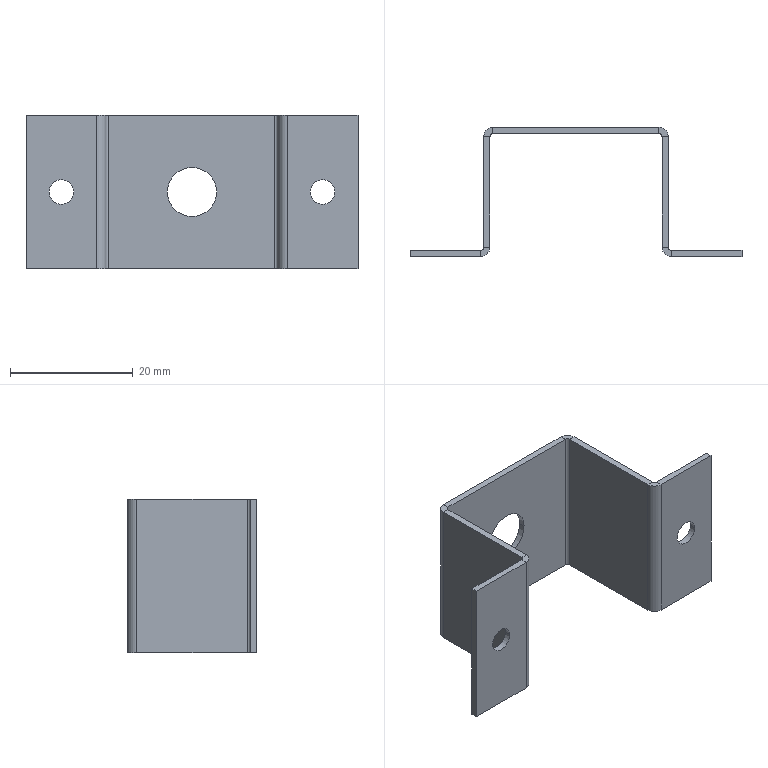Part | SolidWorks | features ICE 2, FlatPattern 1, SMBaseFlange 1, SheetMetal 1 | 1 solid | 44 faces | box 54 x 21 x 25 mm | volume 2232 mm3 | plane 30 | cylinder 14 | commonest cylinder face diameters 1 x4 3 x4 4 x4 8 x2
STEP:
#1=CARTESIAN_POINT('',(23.25,-21.,12.5));
#2=VERTEX_POINT('',#1);
#3=CARTESIAN_POINT('',(19.25,-21.,12.5));
#4=VERTEX_POINT('',#3);
#5=CARTESIAN_POINT('',(21.25,-21.,12.5));
#6=DIRECTION('',(0.,1.,0.));
#7=DIRECTION('',(-1.,0.,0.));
#8=AXIS2_PLACEMENT_3D('',#5,#6,#7);
#9=CIRCLE('',#8,2.);
#10=EDGE_CURVE('',#2,#4,#9,.T.);
#11=ORIENTED_EDGE('',*,*,#10,.F.);
#12=CARTESIAN_POINT('',(23.25,-20.,12.5));
#13=VERTEX_POINT('',#12);
#14=CARTESIAN_POINT('',(23.25,-21.,12.5));
#15=DIRECTION('',(0.,1.,0.));
#16=VECTOR('',#15,1000.);
#17=LINE('',#14,#16);
#18=EDGE_CURVE('',#2,#13,#17,.T.);
#19=ORIENTED_EDGE('',*,*,#18,.T.);
#20=CARTESIAN_POINT('',(19.25,-20.,12.5));
#21=VERTEX_POINT('',#20);
#22=CARTESIAN_POINT('',(21.25,-20.,12.5));
#23=DIRECTION('',(0.,1.,0.));
#24=DIRECTION('',(-1.,0.,0.));
#25=AXIS2_PLACEMENT_3D('',#22,#23,#24);
#26=CIRCLE('',#25,2.);
#27=EDGE_CURVE('',#13,#21,#26,.T.);
#28=ORIENTED_EDGE('',*,*,#27,.T.);
#29=CARTESIAN_POINT('',(19.25,-21.,12.5));
#30=DIRECTION('',(0.,1.,0.));
#31=VECTOR('',#30,1000.);
#32=LINE('',#29,#31);
#33=EDGE_CURVE('',#4,#21,#32,.T.);
#34=ORIENTED_EDGE('',*,*,#33,.F.);
#35=EDGE_LOOP('',(#11,#19,#28,#34));
#36=FACE_OUTER_BOUND('',#35,.T.);
#37=CARTESIAN_POINT('',(21.25,-21.,12.5));
#38=DIRECTION('',(0.,1.,0.));
#39=DIRECTION('',(-1.,0.,0.));
#40=AXIS2_PLACEMENT_3D('',#37,#38,#39);
#41=CYLINDRICAL_SURFACE('',#40,2.);
#42=ADVANCED_FACE('',(#36),#41,.F.);
#43=CARTESIAN_POINT('',(-19.25,-21.,12.5));
#44=VERTEX_POINT('',#43);
#45=CARTESIAN_POINT('',(-23.25,-21.,12.5));
#46=VERTEX_POINT('',#45);
#47=CARTESIAN_POINT('',(-21.25,-21.,12.5));
#48=DIRECTION('',(0.,1.,0.));
#49=DIRECTION('',(-1.,0.,0.));
#50=AXIS2_PLACEMENT_3D('',#47,#48,#49);
#51=CIRCLE('',#50,2.);
#52=EDGE_CURVE('',#44,#46,#51,.T.);
#53=ORIENTED_EDGE('',*,*,#52,.F.);
#54=CARTESIAN_POINT('',(-19.25,-20.,12.5));
#55=VERTEX_POINT('',#54);
#56=CARTESIAN_POINT('',(-19.25,-21.,12.5));
#57=DIRECTION('',(0.,1.,0.));
#58=VECTOR('',#57,1000.);
#59=LINE('',#56,#58);
#60=EDGE_CURVE('',#44,#55,#59,.T.);
#61=ORIENTED_EDGE('',*,*,#60,.T.);
#62=CARTESIAN_POINT('',(-23.25,-20.,12.5));
#63=VERTEX_POINT('',#62);
#64=CARTESIAN_POINT('',(-21.25,-20.,12.5));
#65=DIRECTION('',(0.,1.,0.));
#66=DIRECTION('',(-1.,0.,0.));
#67=AXIS2_PLACEMENT_3D('',#64,#65,#66);
#68=CIRCLE('',#67,2.);
#69=EDGE_CURVE('',#55,#63,#68,.T.);
#70=ORIENTED_EDGE('',*,*,#69,.T.);
#71=CARTESIAN_POINT('',(-23.25,-21.,12.5));
#72=DIRECTION('',(0.,1.,0.));
#73=VECTOR('',#72,1000.);
#74=LINE('',#71,#73);
#75=EDGE_CURVE('',#46,#63,#74,.T.);
#76=ORIENTED_EDGE('',*,*,#75,.F.);
#77=EDGE_LOOP('',(#53,#61,#70,#76));
#78=FACE_OUTER_BOUND('',#77,.T.);
#79=CARTESIAN_POINT('',(-21.25,-21.,12.5));
#80=DIRECTION('',(0.,1.,0.));
#81=DIRECTION('',(-1.,0.,0.));
#82=AXIS2_PLACEMENT_3D('',#79,#80,#81);
#83=CYLINDRICAL_SURFACE('',#82,2.);
#84=ADVANCED_FACE('',(#78),#83,.F.);
#85=CARTESIAN_POINT('',(4.,-1.,12.5));
#86=VERTEX_POINT('',#85);
#87=CARTESIAN_POINT('',(-4.,-1.,12.5));
#88=VERTEX_POINT('',#87);
#89=CARTESIAN_POINT('',(0.,-1.,12.5));
#90=DIRECTION('',(0.,1.,0.));
#91=DIRECTION('',(-1.,0.,0.));
#92=AXIS2_PLACEMENT_3D('',#89,#90,#91);
#93=CIRCLE('',#92,4.);
#94=EDGE_CURVE('',#86,#88,#93,.T.);
#95=ORIENTED_EDGE('',*,*,#94,.F.);
#96=CARTESIAN_POINT('',(4.,0.,12.5));
#97=VERTEX_POINT('',#96);
#98=CARTESIAN_POINT('',(4.,-21.,12.5));
#99=DIRECTION('',(0.,1.,0.));
#100=VECTOR('',#99,1000.);
#101=LINE('',#98,#100);
#102=EDGE_CURVE('',#86,#97,#101,.T.);
#103=ORIENTED_EDGE('',*,*,#102,.T.);
#104=CARTESIAN_POINT('',(-4.,0.,12.5));
#105=VERTEX_POINT('',#104);
#106=CARTESIAN_POINT('',(0.,0.,12.5));
#107=DIRECTION('',(0.,1.,0.));
#108=DIRECTION('',(-1.,0.,0.));
#109=AXIS2_PLACEMENT_3D('',#106,#107,#108);
#110=CIRCLE('',#109,4.);
#111=EDGE_CURVE('',#97,#105,#110,.T.);
#112=ORIENTED_EDGE('',*,*,#111,.T.);
#113=CARTESIAN_POINT('',(-4.,-21.,12.5));
#114=DIRECTION('',(0.,1.,0.));
#115=VECTOR('',#114,1000.);
#116=LINE('',#113,#115);
#117=EDGE_CURVE('',#88,#105,#116,.T.);
#118=ORIENTED_EDGE('',*,*,#117,.F.);
#119=EDGE_LOOP('',(#95,#103,#112,#118));
#120=FACE_OUTER_BOUND('',#119,.T.);
#121=CARTESIAN_POINT('',(0.,-21.,12.5));
#122=DIRECTION('',(0.,1.,0.));
#123=DIRECTION('',(-1.,0.,0.));
#124=AXIS2_PLACEMENT_3D('',#121,#122,#123);
#125=CYLINDRICAL_SURFACE('',#124,4.);
#126=ADVANCED_FACE('',(#120),#125,.F.);
#127=CARTESIAN_POINT('',(-15.,-19.5,25.));
#128=VERTEX_POINT('',#127);
#129=CARTESIAN_POINT('',(-14.,-19.5,25.));
#130=VERTEX_POINT('',#129);
#131=CARTESIAN_POINT('',(-15.,-19.5,25.));
#132=DIRECTION('',(1.,0.,0.));
#133=VECTOR('',#132,1000.);
#134=LINE('',#131,#133);
#135=EDGE_CURVE('',#128,#130,#134,.T.);
#136=ORIENTED_EDGE('',*,*,#135,.F.);
#137=CARTESIAN_POINT('',(-15.5,-20.,25.));
#138=VERTEX_POINT('',#137);
#139=CARTESIAN_POINT('',(-15.5,-19.5,25.));
#140=DIRECTION('',(0.,0.,1.));
#141=DIRECTION('',(-1.,0.,0.));
#142=AXIS2_PLACEMENT_3D('',#139,#140,#141);
#143=CIRCLE('',#142,0.5);
#144=EDGE_CURVE('',#138,#128,#143,.T.);
#145=ORIENTED_EDGE('',*,*,#144,.F.);
#146=CARTESIAN_POINT('',(-15.5,-21.,25.));
#147=VERTEX_POINT('',#146);
#148=CARTESIAN_POINT('',(-15.5,-21.,25.));
#149=DIRECTION('',(0.,1.,0.));
#150=VECTOR('',#149,1000.);
#151=LINE('',#148,#150);
#152=EDGE_CURVE('',#147,#138,#151,.T.);
#153=ORIENTED_EDGE('',*,*,#152,.F.);
#154=CARTESIAN_POINT('',(-15.5,-19.5,25.));
#155=DIRECTION('',(0.,0.,1.));
#156=DIRECTION('',(1.,0.,0.));
#157=AXIS2_PLACEMENT_3D('',#154,#155,#156);
#158=CIRCLE('',#157,1.5);
#159=EDGE_CURVE('',#147,#130,#158,.T.);
#160=ORIENTED_EDGE('',*,*,#159,.T.);
#161=EDGE_LOOP('',(#136,#145,#153,#160));
#162=FACE_OUTER_BOUND('',#161,.T.);
#163=CARTESIAN_POINT('',(-15.,-19.5,25.));
#164=DIRECTION('',(0.,0.,1.));
#165=DIRECTION('',(1.,0.,0.));
#166=AXIS2_PLACEMENT_3D('',#163,#164,#165);
#167=PLANE('',#166);
#168=ADVANCED_FACE('',(#162),#167,.T.);
#169=CARTESIAN_POINT('',(-15.,-1.5,25.));
#170=VERTEX_POINT('',#169);
#171=CARTESIAN_POINT('',(-15.,0.,25.));
#172=DIRECTION('',(0.,1.,0.));
#173=VECTOR('',#172,1000.);
#174=LINE('',#171,#173);
#175=EDGE_CURVE('',#128,#170,#174,.T.);
#176=ORIENTED_EDGE('',*,*,#175,.F.);
#177=ORIENTED_EDGE('',*,*,#135,.T.);
#178=CARTESIAN_POINT('',(-14.,-1.5,25.));
#179=VERTEX_POINT('',#178);
#180=CARTESIAN_POINT('',(-14.,0.,25.));
#181=DIRECTION('',(0.,1.,0.));
#182=VECTOR('',#181,1000.);
#183=LINE('',#180,#182);
#184=EDGE_CURVE('',#130,#179,#183,.T.);
#185=ORIENTED_EDGE('',*,*,#184,.T.);
#186=CARTESIAN_POINT('',(-14.,-1.5,25.));
#187=DIRECTION('',(-1.,0.,0.));
#188=VECTOR('',#187,1000.);
#189=LINE('',#186,#188);
#190=EDGE_CURVE('',#179,#170,#189,.T.);
#191=ORIENTED_EDGE('',*,*,#190,.T.);
#192=EDGE_LOOP('',(#176,#177,#185,#191));
#193=FACE_OUTER_BOUND('',#192,.T.);
#194=CARTESIAN_POINT('',(-15.5,-21.,25.));
#195=DIRECTION('',(0.,0.,1.));
#196=DIRECTION('',(1.,0.,0.));
#197=AXIS2_PLACEMENT_3D('',#194,#195,#196);
#198=PLANE('',#197);
#199=ADVANCED_FACE('',(#193),#198,.T.);
#200=CARTESIAN_POINT('',(-15.5,-20.,0.));
#201=VERTEX_POINT('',#200);
#202=CARTESIAN_POINT('',(-15.5,-21.,0.));
#203=VERTEX_POINT('',#202);
#204=CARTESIAN_POINT('',(-15.5,-20.,0.));
#205=DIRECTION('',(0.,-1.,0.));
#206=VECTOR('',#205,1000.);
#207=LINE('',#204,#206);
#208=EDGE_CURVE('',#201,#203,#207,.T.);
#209=ORIENTED_EDGE('',*,*,#208,.F.);
#210=CARTESIAN_POINT('',(-15.,-19.5,0.));
#211=VERTEX_POINT('',#210);
#212=CARTESIAN_POINT('',(-15.5,-19.5,0.));
#213=DIRECTION('',(0.,0.,1.));
#214=DIRECTION('',(-1.,0.,0.));
#215=AXIS2_PLACEMENT_3D('',#212,#213,#214);
#216=CIRCLE('',#215,0.5);
#217=EDGE_CURVE('',#201,#211,#216,.T.);
#218=ORIENTED_EDGE('',*,*,#217,.T.);
#219=CARTESIAN_POINT('',(-14.,-19.5,0.));
#220=VERTEX_POINT('',#219);
#221=CARTESIAN_POINT('',(-14.,-19.5,0.));
#222=DIRECTION('',(-1.,0.,0.));
#223=VECTOR('',#222,1000.);
#224=LINE('',#221,#223);
#225=EDGE_CURVE('',#220,#211,#224,.T.);
#226=ORIENTED_EDGE('',*,*,#225,.F.);
#227=CARTESIAN_POINT('',(-15.5,-19.5,0.));
#228=DIRECTION('',(0.,0.,1.));
#229=DIRECTION('',(1.,0.,0.));
#230=AXIS2_PLACEMENT_3D('',#227,#228,#229);
#231=CIRCLE('',#230,1.5);
#232=EDGE_CURVE('',#203,#220,#231,.T.);
#233=ORIENTED_EDGE('',*,*,#232,.F.);
#234=EDGE_LOOP('',(#209,#218,#226,#233));
#235=FACE_OUTER_BOUND('',#234,.T.);
#236=CARTESIAN_POINT('',(-15.5,-20.,0.));
#237=DIRECTION('',(0.,0.,-1.));
#238=DIRECTION('',(-1.,0.,0.));
#239=AXIS2_PLACEMENT_3D('',#236,#237,#238);
#240=PLANE('',#239);
#241=ADVANCED_FACE('',(#235),#240,.T.);
#242=CARTESIAN_POINT('',(-27.,-20.,0.));
#243=VERTEX_POINT('',#242);
#244=CARTESIAN_POINT('',(-15.,-20.,0.));
#245=DIRECTION('',(1.,0.,0.));
#246=VECTOR('',#245,1000.);
#247=LINE('',#244,#246);
#248=EDGE_CURVE('',#243,#201,#247,.T.);
#249=ORIENTED_EDGE('',*,*,#248,.T.);
#250=ORIENTED_EDGE('',*,*,#208,.T.);
#251=CARTESIAN_POINT('',(-27.,-21.,0.));
#252=VERTEX_POINT('',#251);
#253=CARTESIAN_POINT('',(-15.,-21.,0.));
#254=DIRECTION('',(1.,0.,0.));
#255=VECTOR('',#254,1000.);
#256=LINE('',#253,#255);
#257=EDGE_CURVE('',#252,#203,#256,.T.);
#258=ORIENTED_EDGE('',*,*,#257,.F.);
#259=CARTESIAN_POINT('',(-27.,-21.,0.));
#260=DIRECTION('',(0.,1.,0.));
#261=VECTOR('',#260,1000.);
#262=LINE('',#259,#261);
#263=EDGE_CURVE('',#252,#243,#262,.T.);
#264=ORIENTED_EDGE('',*,*,#263,.T.);
#265=EDGE_LOOP('',(#249,#250,#258,#264));
#266=FACE_OUTER_BOUND('',#265,.T.);
#267=CARTESIAN_POINT('',(-14.,-19.5,0.));
#268=DIRECTION('',(0.,0.,-1.));
#269=DIRECTION('',(-1.,0.,0.));
#270=AXIS2_PLACEMENT_3D('',#267,#268,#269);
#271=PLANE('',#270);
#272=ADVANCED_FACE('',(#266),#271,.T.);
#273=CARTESIAN_POINT('',(-13.5,0.,25.));
#274=VERTEX_POINT('',#273);
#275=CARTESIAN_POINT('',(-13.5,-1.,25.));
#276=VERTEX_POINT('',#275);
#277=CARTESIAN_POINT('',(-13.5,0.,25.));
#278=DIRECTION('',(0.,-1.,0.));
#279=VECTOR('',#278,1000.);
#280=LINE('',#277,#279);
#281=EDGE_CURVE('',#274,#276,#280,.T.);
#282=ORIENTED_EDGE('',*,*,#281,.F.);
#283=CARTESIAN_POINT('',(-13.5,-1.5,25.));
#284=DIRECTION('',(0.,0.,-1.));
#285=DIRECTION('',(1.,0.,0.));
#286=AXIS2_PLACEMENT_3D('',#283,#284,#285);
#287=CIRCLE('',#286,1.5);
#288=EDGE_CURVE('',#170,#274,#287,.T.);
#289=ORIENTED_EDGE('',*,*,#288,.F.);
#290=ORIENTED_EDGE('',*,*,#190,.F.);
#291=CARTESIAN_POINT('',(-13.5,-1.5,25.));
#292=DIRECTION('',(0.,0.,-1.));
#293=DIRECTION('',(1.,0.,0.));
#294=AXIS2_PLACEMENT_3D('',#291,#292,#293);
#295=CIRCLE('',#294,0.5);
#296=EDGE_CURVE('',#179,#276,#295,.T.);
#297=ORIENTED_EDGE('',*,*,#296,.T.);
#298=EDGE_LOOP('',(#282,#289,#290,#297));
#299=FACE_OUTER_BOUND('',#298,.T.);
#300=CARTESIAN_POINT('',(-13.5,0.,25.));
#301=DIRECTION('',(0.,0.,1.));
#302=DIRECTION('',(1.,0.,0.));
#303=AXIS2_PLACEMENT_3D('',#300,#301,#302);
#304=PLANE('',#303);
#305=ADVANCED_FACE('',(#299),#304,.T.);
#306=CARTESIAN_POINT('',(13.5,0.,25.));
#307=VERTEX_POINT('',#306);
#308=CARTESIAN_POINT('',(-15.,0.,25.));
#309=DIRECTION('',(1.,0.,0.));
#310=VECTOR('',#309,1000.);
#311=LINE('',#308,#310);
#312=EDGE_CURVE('',#274,#307,#311,.T.);
#313=ORIENTED_EDGE('',*,*,#312,.F.);
#314=ORIENTED_EDGE('',*,*,#281,.T.);
#315=CARTESIAN_POINT('',(13.5,-1.,25.));
#316=VERTEX_POINT('',#315);
#317=CARTESIAN_POINT('',(-15.,-1.,25.));
#318=DIRECTION('',(1.,0.,0.));
#319=VECTOR('',#318,1000.);
#320=LINE('',#317,#319);
#321=EDGE_CURVE('',#276,#316,#320,.T.);
#322=ORIENTED_EDGE('',*,*,#321,.T.);
#323=CARTESIAN_POINT('',(13.5,-1.,25.));
#324=DIRECTION('',(0.,1.,0.));
#325=VECTOR('',#324,1000.);
#326=LINE('',#323,#325);
#327=EDGE_CURVE('',#316,#307,#326,.T.);
#328=ORIENTED_EDGE('',*,*,#327,.T.);
#329=EDGE_LOOP('',(#313,#314,#322,#328));
#330=FACE_OUTER_BOUND('',#329,.T.);
#331=CARTESIAN_POINT('',(-14.,-1.5,25.));
#332=DIRECTION('',(0.,0.,1.));
#333=DIRECTION('',(1.,0.,0.));
#334=AXIS2_PLACEMENT_3D('',#331,#332,#333);
#335=PLANE('',#334);
#336=ADVANCED_FACE('',(#330),#335,.T.);
#337=CARTESIAN_POINT('',(-15.,-1.5,0.));
#338=VERTEX_POINT('',#337);
#339=CARTESIAN_POINT('',(-14.,-1.5,0.));
#340=VERTEX_POINT('',#339);
#341=CARTESIAN_POINT('',(-15.,-1.5,0.));
#342=DIRECTION('',(1.,0.,0.));
#343=VECTOR('',#342,1000.);
#344=LINE('',#341,#343);
#345=EDGE_CURVE('',#338,#340,#344,.T.);
#346=ORIENTED_EDGE('',*,*,#345,.F.);
#347=CARTESIAN_POINT('',(-13.5,0.,0.));
#348=VERTEX_POINT('',#347);
#349=CARTESIAN_POINT('',(-13.5,-1.5,0.));
#350=DIRECTION('',(0.,0.,-1.));
#351=DIRECTION('',(1.,0.,0.));
#352=AXIS2_PLACEMENT_3D('',#349,#350,#351);
#353=CIRCLE('',#352,1.5);
#354=EDGE_CURVE('',#338,#348,#353,.T.);
#355=ORIENTED_EDGE('',*,*,#354,.T.);
#356=CARTESIAN_POINT('',(-13.5,-1.,0.));
#357=VERTEX_POINT('',#356);
#358=CARTESIAN_POINT('',(-13.5,-1.,0.));
#359=DIRECTION('',(0.,1.,0.));
#360=VECTOR('',#359,1000.);
#361=LINE('',#358,#360);
#362=EDGE_CURVE('',#357,#348,#361,.T.);
#363=ORIENTED_EDGE('',*,*,#362,.F.);
#364=CARTESIAN_POINT('',(-13.5,-1.5,0.));
#365=DIRECTION('',(0.,0.,-1.));
#366=DIRECTION('',(1.,0.,0.));
#367=AXIS2_PLACEMENT_3D('',#364,#365,#366);
#368=CIRCLE('',#367,0.5);
#369=EDGE_CURVE('',#340,#357,#368,.T.);
#370=ORIENTED_EDGE('',*,*,#369,.F.);
#371=EDGE_LOOP('',(#346,#355,#363,#370));
#372=FACE_OUTER_BOUND('',#371,.T.);
#373=CARTESIAN_POINT('',(-15.,-1.5,0.));
#374=DIRECTION('',(0.,0.,-1.));
#375=DIRECTION('',(-1.,0.,0.));
#376=AXIS2_PLACEMENT_3D('',#373,#374,#375);
#377=PLANE('',#376);
#378=ADVANCED_FACE('',(#372),#377,.T.);
#379=CARTESIAN_POINT('',(-15.,0.,0.));
#380=DIRECTION('',(0.,1.,0.));
#381=VECTOR('',#380,1000.);
#382=LINE('',#379,#381);
#383=EDGE_CURVE('',#211,#338,#382,.T.);
#384=ORIENTED_EDGE('',*,*,#383,.T.);
#385=ORIENTED_EDGE('',*,*,#345,.T.);
#386=CARTESIAN_POINT('',(-14.,0.,0.));
#387=DIRECTION('',(0.,1.,0.));
#388=VECTOR('',#387,1000.);
#389=LINE('',#386,#388);
#390=EDGE_CURVE('',#220,#340,#389,.T.);
#391=ORIENTED_EDGE('',*,*,#390,.F.);
#392=ORIENTED_EDGE('',*,*,#225,.T.);
#393=EDGE_LOOP('',(#384,#385,#391,#392));
#394=FACE_OUTER_BOUND('',#393,.T.);
#395=CARTESIAN_POINT('',(-13.5,-1.,0.));
#396=DIRECTION('',(0.,0.,-1.));
#397=DIRECTION('',(-1.,0.,0.));
#398=AXIS2_PLACEMENT_3D('',#395,#396,#397);
#399=PLANE('',#398);
#400=ADVANCED_FACE('',(#394),#399,.T.);
#401=CARTESIAN_POINT('',(15.,-1.5,25.));
#402=VERTEX_POINT('',#401);
#403=CARTESIAN_POINT('',(14.,-1.5,25.));
#404=VERTEX_POINT('',#403);
#405=CARTESIAN_POINT('',(15.,-1.5,25.));
#406=DIRECTION('',(-1.,0.,0.));
#407=VECTOR('',#406,1000.);
#408=LINE('',#405,#407);
#409=EDGE_CURVE('',#402,#404,#408,.T.);
#410=ORIENTED_EDGE('',*,*,#409,.F.);
#411=CARTESIAN_POINT('',(13.5,-1.5,25.));
#412=DIRECTION('',(0.,0.,-1.));
#413=DIRECTION('',(1.,0.,0.));
#414=AXIS2_PLACEMENT_3D('',#411,#412,#413);
#415=CIRCLE('',#414,1.5);
#416=EDGE_CURVE('',#307,#402,#415,.T.);
#417=ORIENTED_EDGE('',*,*,#416,.F.);
#418=ORIENTED_EDGE('',*,*,#327,.F.);
#419=CARTESIAN_POINT('',(13.5,-1.5,25.));
#420=DIRECTION('',(0.,0.,-1.));
#421=DIRECTION('',(1.,0.,0.));
#422=AXIS2_PLACEMENT_3D('',#419,#420,#421);
#423=CIRCLE('',#422,0.5);
#424=EDGE_CURVE('',#316,#404,#423,.T.);
#425=ORIENTED_EDGE('',*,*,#424,.T.);
#426=EDGE_LOOP('',(#410,#417,#418,#425));
#427=FACE_OUTER_BOUND('',#426,.T.);
#428=CARTESIAN_POINT('',(15.,-1.5,25.));
#429=DIRECTION('',(0.,0.,1.));
#430=DIRECTION('',(1.,0.,0.));
#431=AXIS2_PLACEMENT_3D('',#428,#429,#430);
#432=PLANE('',#431);
#433=ADVANCED_FACE('',(#427),#432,.T.);
#434=CARTESIAN_POINT('',(15.,-19.5,25.));
#435=VERTEX_POINT('',#434);
#436=CARTESIAN_POINT('',(15.,0.,25.));
#437=DIRECTION('',(0.,-1.,0.));
#438=VECTOR('',#437,1000.);
#439=LINE('',#436,#438);
#440=EDGE_CURVE('',#402,#435,#439,.T.);
#441=ORIENTED_EDGE('',*,*,#440,.F.);
#442=ORIENTED_EDGE('',*,*,#409,.T.);
#443=CARTESIAN_POINT('',(14.,-19.5,25.));
#444=VERTEX_POINT('',#443);
#445=CARTESIAN_POINT('',(14.,0.,25.));
#446=DIRECTION('',(0.,-1.,0.));
#447=VECTOR('',#446,1000.);
#448=LINE('',#445,#447);
#449=EDGE_CURVE('',#404,#444,#448,.T.);
#450=ORIENTED_EDGE('',*,*,#449,.T.);
#451=CARTESIAN_POINT('',(14.,-19.5,25.));
#452=DIRECTION('',(1.,0.,0.));
#453=VECTOR('',#452,1000.);
#454=LINE('',#451,#453);
#455=EDGE_CURVE('',#444,#435,#454,.T.);
#456=ORIENTED_EDGE('',*,*,#455,.T.);
#457=EDGE_LOOP('',(#441,#442,#450,#456));
#458=FACE_OUTER_BOUND('',#457,.T.);
#459=CARTESIAN_POINT('',(13.5,-1.,25.));
#460=DIRECTION('',(0.,0.,1.));
#461=DIRECTION('',(1.,0.,0.));
#462=AXIS2_PLACEMENT_3D('',#459,#460,#461);
#463=PLANE('',#462);
#464=ADVANCED_FACE('',(#458),#463,.T.);
#465=CARTESIAN_POINT('',(13.5,0.,0.));
#466=VERTEX_POINT('',#465);
#467=CARTESIAN_POINT('',(13.5,-1.,0.));
#468=VERTEX_POINT('',#467);
#469=CARTESIAN_POINT('',(13.5,0.,0.));
#470=DIRECTION('',(0.,-1.,0.));
#471=VECTOR('',#470,1000.);
#472=LINE('',#469,#471);
#473=EDGE_CURVE('',#466,#468,#472,.T.);
#474=ORIENTED_EDGE('',*,*,#473,.F.);
#475=CARTESIAN_POINT('',(15.,-1.5,0.));
#476=VERTEX_POINT('',#475);
#477=CARTESIAN_POINT('',(13.5,-1.5,0.));
#478=DIRECTION('',(0.,0.,-1.));
#479=DIRECTION('',(1.,0.,0.));
#480=AXIS2_PLACEMENT_3D('',#477,#478,#479);
#481=CIRCLE('',#480,1.5);
#482=EDGE_CURVE('',#466,#476,#481,.T.);
#483=ORIENTED_EDGE('',*,*,#482,.T.);
#484=CARTESIAN_POINT('',(14.,-1.5,0.));
#485=VERTEX_POINT('',#484);
#486=CARTESIAN_POINT('',(14.,-1.5,0.));
#487=DIRECTION('',(1.,0.,0.));
#488=VECTOR('',#487,1000.);
#489=LINE('',#486,#488);
#490=EDGE_CURVE('',#485,#476,#489,.T.);
#491=ORIENTED_EDGE('',*,*,#490,.F.);
#492=CARTESIAN_POINT('',(13.5,-1.5,0.));
#493=DIRECTION('',(0.,0.,-1.));
#494=DIRECTION('',(1.,0.,0.));
#495=AXIS2_PLACEMENT_3D('',#492,#493,#494);
#496=CIRCLE('',#495,0.5);
#497=EDGE_CURVE('',#468,#485,#496,.T.);
#498=ORIENTED_EDGE('',*,*,#497,.F.);
#499=EDGE_LOOP('',(#474,#483,#491,#498));
#500=FACE_OUTER_BOUND('',#499,.T.);
#501=CARTESIAN_POINT('',(13.5,0.,0.));
#502=DIRECTION('',(0.,0.,-1.));
#503=DIRECTION('',(-1.,0.,0.));
#504=AXIS2_PLACEMENT_3D('',#501,#502,#503);
#505=PLANE('',#504);
#506=ADVANCED_FACE('',(#500),#505,.T.);
#507=CARTESIAN_POINT('',(-15.,0.,0.));
#508=DIRECTION('',(1.,0.,0.));
#509=VECTOR('',#508,1000.);
#510=LINE('',#507,#509);
#511=EDGE_CURVE('',#348,#466,#510,.T.);
#512=ORIENTED_EDGE('',*,*,#511,.T.);
#513=ORIENTED_EDGE('',*,*,#473,.T.);
#514=CARTESIAN_POINT('',(-15.,-1.,0.));
#515=DIRECTION('',(1.,0.,0.));
#516=VECTOR('',#515,1000.);
#517=LINE('',#514,#516);
#518=EDGE_CURVE('',#357,#468,#517,.T.);
#519=ORIENTED_EDGE('',*,*,#518,.F.);
#520=ORIENTED_EDGE('',*,*,#362,.T.);
#521=EDGE_LOOP('',(#512,#513,#519,#520));
#522=FACE_OUTER_BOUND('',#521,.T.);
#523=CARTESIAN_POINT('',(14.,-1.5,0.));
#524=DIRECTION('',(0.,0.,-1.));
#525=DIRECTION('',(-1.,0.,0.));
#526=AXIS2_PLACEMENT_3D('',#523,#524,#525);
#527=PLANE('',#526);
#528=ADVANCED_FACE('',(#522),#527,.T.);
#529=CARTESIAN_POINT('',(15.5,-20.,25.));
#530=VERTEX_POINT('',#529);
#531=CARTESIAN_POINT('',(15.5,-21.,25.));
#532=VERTEX_POINT('',#531);
#533=CARTESIAN_POINT('',(15.5,-20.,25.));
#534=DIRECTION('',(0.,-1.,0.));
#535=VECTOR('',#534,1000.);
#536=LINE('',#533,#535);
#537=EDGE_CURVE('',#530,#532,#536,.T.);
#538=ORIENTED_EDGE('',*,*,#537,.F.);
#539=CARTESIAN_POINT('',(15.5,-19.5,25.));
#540=DIRECTION('',(0.,0.,1.));
#541=DIRECTION('',(-1.,0.,0.));
#542=AXIS2_PLACEMENT_3D('',#539,#540,#541);
#543=CIRCLE('',#542,0.5);
#544=EDGE_CURVE('',#435,#530,#543,.T.);
#545=ORIENTED_EDGE('',*,*,#544,.F.);
#546=ORIENTED_EDGE('',*,*,#455,.F.);
#547=CARTESIAN_POINT('',(15.5,-19.5,25.));
#548=DIRECTION('',(0.,0.,1.));
#549=DIRECTION('',(1.,0.,0.));
#550=AXIS2_PLACEMENT_3D('',#547,#548,#549);
#551=CIRCLE('',#550,1.5);
#552=EDGE_CURVE('',#444,#532,#551,.T.);
#553=ORIENTED_EDGE('',*,*,#552,.T.);
#554=EDGE_LOOP('',(#538,#545,#546,#553));
#555=FACE_OUTER_BOUND('',#554,.T.);
#556=CARTESIAN_POINT('',(15.5,-20.,25.));
#557=DIRECTION('',(0.,0.,1.));
#558=DIRECTION('',(1.,0.,0.));
#559=AXIS2_PLACEMENT_3D('',#556,#557,#558);
#560=PLANE('',#559);
#561=ADVANCED_FACE('',(#555),#560,.T.);
#562=CARTESIAN_POINT('',(27.,-20.,25.));
#563=VERTEX_POINT('',#562);
#564=CARTESIAN_POINT('',(15.,-20.,25.));
#565=DIRECTION('',(1.,0.,0.));
#566=VECTOR('',#565,1000.);
#567=LINE('',#564,#566);
#568=EDGE_CURVE('',#530,#563,#567,.T.);
#569=ORIENTED_EDGE('',*,*,#568,.F.);
#570=ORIENTED_EDGE('',*,*,#537,.T.);
#571=CARTESIAN_POINT('',(27.,-21.,25.));
#572=VERTEX_POINT('',#571);
#573=CARTESIAN_POINT('',(15.,-21.,25.));
#574=DIRECTION('',(1.,0.,0.));
#575=VECTOR('',#574,1000.);
#576=LINE('',#573,#575);
#577=EDGE_CURVE('',#532,#572,#576,.T.);
#578=ORIENTED_EDGE('',*,*,#577,.T.);
#579=CARTESIAN_POINT('',(27.,-20.,25.));
#580=DIRECTION('',(0.,-1.,0.));
#581=VECTOR('',#580,1000.);
#582=LINE('',#579,#581);
#583=EDGE_CURVE('',#563,#572,#582,.T.);
#584=ORIENTED_EDGE('',*,*,#583,.F.);
#585=EDGE_LOOP('',(#569,#570,#578,#584));
#586=FACE_OUTER_BOUND('',#585,.T.);
#587=CARTESIAN_POINT('',(14.,-19.5,25.));
#588=DIRECTION('',(0.,0.,1.));
#589=DIRECTION('',(1.,0.,0.));
#590=AXIS2_PLACEMENT_3D('',#587,#588,#589);
#591=PLANE('',#590);
#592=ADVANCED_FACE('',(#586),#591,.T.);
#593=CARTESIAN_POINT('',(15.,-19.5,0.));
#594=VERTEX_POINT('',#593);
#595=CARTESIAN_POINT('',(14.,-19.5,0.));
#596=VERTEX_POINT('',#595);
#597=CARTESIAN_POINT('',(15.,-19.5,0.));
#598=DIRECTION('',(-1.,0.,0.));
#599=VECTOR('',#598,1000.);
#600=LINE('',#597,#599);
#601=EDGE_CURVE('',#594,#596,#600,.T.);
#602=ORIENTED_EDGE('',*,*,#601,.F.);
#603=CARTESIAN_POINT('',(15.5,-20.,0.));
#604=VERTEX_POINT('',#603);
#605=CARTESIAN_POINT('',(15.5,-19.5,0.));
#606=DIRECTION('',(0.,0.,1.));
#607=DIRECTION('',(-1.,0.,0.));
#608=AXIS2_PLACEMENT_3D('',#605,#606,#607);
#609=CIRCLE('',#608,0.5);
#610=EDGE_CURVE('',#594,#604,#609,.T.);
#611=ORIENTED_EDGE('',*,*,#610,.T.);
#612=CARTESIAN_POINT('',(15.5,-21.,0.));
#613=VERTEX_POINT('',#612);
#614=CARTESIAN_POINT('',(15.5,-21.,0.));
#615=DIRECTION('',(0.,1.,0.));
#616=VECTOR('',#615,1000.);
#617=LINE('',#614,#616);
#618=EDGE_CURVE('',#613,#604,#617,.T.);
#619=ORIENTED_EDGE('',*,*,#618,.F.);
#620=CARTESIAN_POINT('',(15.5,-19.5,0.));
#621=DIRECTION('',(0.,0.,1.));
#622=DIRECTION('',(1.,0.,0.));
#623=AXIS2_PLACEMENT_3D('',#620,#621,#622);
#624=CIRCLE('',#623,1.5);
#625=EDGE_CURVE('',#596,#613,#624,.T.);
#626=ORIENTED_EDGE('',*,*,#625,.F.);
#627=EDGE_LOOP('',(#602,#611,#619,#626));
#628=FACE_OUTER_BOUND('',#627,.T.);
#629=CARTESIAN_POINT('',(15.,-19.5,0.));
#630=DIRECTION('',(0.,0.,-1.));
#631=DIRECTION('',(-1.,0.,0.));
#632=AXIS2_PLACEMENT_3D('',#629,#630,#631);
#633=PLANE('',#632);
#634=ADVANCED_FACE('',(#628),#633,.T.);
#635=CARTESIAN_POINT('',(15.,0.,0.));
#636=DIRECTION('',(0.,-1.,0.));
#637=VECTOR('',#636,1000.);
#638=LINE('',#635,#637);
#639=EDGE_CURVE('',#476,#594,#638,.T.);
#640=ORIENTED_EDGE('',*,*,#639,.T.);
#641=ORIENTED_EDGE('',*,*,#601,.T.);
#642=CARTESIAN_POINT('',(14.,0.,0.));
#643=DIRECTION('',(0.,-1.,0.));
#644=VECTOR('',#643,1000.);
#645=LINE('',#642,#644);
#646=EDGE_CURVE('',#485,#596,#645,.T.);
#647=ORIENTED_EDGE('',*,*,#646,.F.);
#648=ORIENTED_EDGE('',*,*,#490,.T.);
#649=EDGE_LOOP('',(#640,#641,#647,#648));
#650=FACE_OUTER_BOUND('',#649,.T.);
#651=CARTESIAN_POINT('',(15.5,-21.,0.));
#652=DIRECTION('',(0.,0.,-1.));
#653=DIRECTION('',(-1.,0.,0.));
#654=AXIS2_PLACEMENT_3D('',#651,#652,#653);
#655=PLANE('',#654);
#656=ADVANCED_FACE('',(#650),#655,.T.);
#657=CARTESIAN_POINT('',(21.25,-21.,12.5));
#658=DIRECTION('',(0.,1.,0.));
#659=DIRECTION('',(-1.,0.,0.));
#660=AXIS2_PLACEMENT_3D('',#657,#658,#659);
#661=CIRCLE('',#660,2.);
#662=EDGE_CURVE('',#4,#2,#661,.T.);
#663=ORIENTED_EDGE('',*,*,#662,.T.);
#664=ORIENTED_EDGE('',*,*,#10,.T.);
#665=EDGE_LOOP('',(#663,#664));
#666=FACE_BOUND('',#665,.T.);
#667=CARTESIAN_POINT('',(27.,-21.,0.));
#668=VERTEX_POINT('',#667);
#669=CARTESIAN_POINT('',(15.,-21.,0.));
#670=DIRECTION('',(1.,0.,0.));
#671=VECTOR('',#670,1000.);
#672=LINE('',#669,#671);
#673=EDGE_CURVE('',#613,#668,#672,.T.);
#674=ORIENTED_EDGE('',*,*,#673,.T.);
#675=CARTESIAN_POINT('',(27.,-21.,25.));
#676=DIRECTION('',(0.,0.,-1.));
#677=VECTOR('',#676,1000.);
#678=LINE('',#675,#677);
#679=EDGE_CURVE('',#572,#668,#678,.T.);
#680=ORIENTED_EDGE('',*,*,#679,.F.);
#681=ORIENTED_EDGE('',*,*,#577,.F.);
#682=CARTESIAN_POINT('',(15.5,-21.,25.));
#683=DIRECTION('',(0.,0.,-1.));
#684=VECTOR('',#683,1000.);
#685=LINE('',#682,#684);
#686=EDGE_CURVE('',#532,#613,#685,.T.);
#687=ORIENTED_EDGE('',*,*,#686,.T.);
#688=EDGE_LOOP('',(#674,#680,#681,#687));
#689=FACE_OUTER_BOUND('',#688,.T.);
#690=CARTESIAN_POINT('',(15.,-21.,25.));
#691=DIRECTION('',(0.,1.,0.));
#692=DIRECTION('',(0.,0.,1.));
#693=AXIS2_PLACEMENT_3D('',#690,#691,#692);
#694=PLANE('',#693);
#695=ADVANCED_FACE('',(#666,#689),#694,.F.);
#696=CARTESIAN_POINT('',(27.,-20.,0.));
#697=VERTEX_POINT('',#696);
#698=CARTESIAN_POINT('',(27.,-20.,0.));
#699=DIRECTION('',(0.,-1.,0.));
#700=VECTOR('',#699,1000.);
#701=LINE('',#698,#700);
#702=EDGE_CURVE('',#697,#668,#701,.T.);
#703=ORIENTED_EDGE('',*,*,#702,.F.);
#704=CARTESIAN_POINT('',(27.,-20.,25.));
#705=DIRECTION('',(0.,0.,-1.));
#706=VECTOR('',#705,1000.);
#707=LINE('',#704,#706);
#708=EDGE_CURVE('',#563,#697,#707,.T.);
#709=ORIENTED_EDGE('',*,*,#708,.F.);
#710=ORIENTED_EDGE('',*,*,#583,.T.);
#711=ORIENTED_EDGE('',*,*,#679,.T.);
#712=EDGE_LOOP('',(#703,#709,#710,#711));
#713=FACE_OUTER_BOUND('',#712,.T.);
#714=CARTESIAN_POINT('',(27.,-20.,25.));
#715=DIRECTION('',(1.,0.,0.));
#716=DIRECTION('',(0.,0.,-1.));
#717=AXIS2_PLACEMENT_3D('',#714,#715,#716);
#718=PLANE('',#717);
#719=ADVANCED_FACE('',(#713),#718,.T.);
#720=CARTESIAN_POINT('',(21.25,-20.,12.5));
#721=DIRECTION('',(0.,1.,0.));
#722=DIRECTION('',(-1.,0.,0.));
#723=AXIS2_PLACEMENT_3D('',#720,#721,#722);
#724=CIRCLE('',#723,2.);
#725=EDGE_CURVE('',#21,#13,#724,.T.);
#726=ORIENTED_EDGE('',*,*,#725,.F.);
#727=ORIENTED_EDGE('',*,*,#27,.F.);
#728=EDGE_LOOP('',(#726,#727));
#729=FACE_BOUND('',#728,.T.);
#730=CARTESIAN_POINT('',(15.,-20.,0.));
#731=DIRECTION('',(1.,0.,0.));
#732=VECTOR('',#731,1000.);
#733=LINE('',#730,#732);
#734=EDGE_CURVE('',#604,#697,#733,.T.);
#735=ORIENTED_EDGE('',*,*,#734,.F.);
#736=CARTESIAN_POINT('',(15.5,-20.,25.));
#737=DIRECTION('',(0.,0.,-1.));
#738=VECTOR('',#737,1000.);
#739=LINE('',#736,#738);
#740=EDGE_CURVE('',#530,#604,#739,.T.);
#741=ORIENTED_EDGE('',*,*,#740,.F.);
#742=ORIENTED_EDGE('',*,*,#568,.T.);
#743=ORIENTED_EDGE('',*,*,#708,.T.);
#744=EDGE_LOOP('',(#735,#741,#742,#743));
#745=FACE_OUTER_BOUND('',#744,.T.);
#746=CARTESIAN_POINT('',(15.,-20.,25.));
#747=DIRECTION('',(0.,1.,0.));
#748=DIRECTION('',(0.,0.,1.));
#749=AXIS2_PLACEMENT_3D('',#746,#747,#748);
#750=PLANE('',#749);
#751=ADVANCED_FACE('',(#729,#745),#750,.T.);
#752=ORIENTED_EDGE('',*,*,#610,.F.);
#753=CARTESIAN_POINT('',(15.,-19.5,25.));
#754=DIRECTION('',(0.,0.,-1.));
#755=VECTOR('',#754,1000.);
#756=LINE('',#753,#755);
#757=EDGE_CURVE('',#435,#594,#756,.T.);
#758=ORIENTED_EDGE('',*,*,#757,.F.);
#759=ORIENTED_EDGE('',*,*,#544,.T.);
#760=ORIENTED_EDGE('',*,*,#740,.T.);
#761=EDGE_LOOP('',(#752,#758,#759,#760));
#762=FACE_OUTER_BOUND('',#761,.T.);
#763=CARTESIAN_POINT('',(15.5,-19.5,25.));
#764=DIRECTION('',(0.,0.,-1.));
#765=DIRECTION('',(-1.,0.,0.));
#766=AXIS2_PLACEMENT_3D('',#763,#764,#765);
#767=CYLINDRICAL_SURFACE('',#766,0.5);
#768=ADVANCED_FACE('',(#762),#767,.F.);
#769=ORIENTED_EDGE('',*,*,#639,.F.);
#770=CARTESIAN_POINT('',(15.,-1.5,25.));
#771=DIRECTION('',(0.,0.,-1.));
#772=VECTOR('',#771,1000.);
#773=LINE('',#770,#772);
#774=EDGE_CURVE('',#402,#476,#773,.T.);
#775=ORIENTED_EDGE('',*,*,#774,.F.);
#776=ORIENTED_EDGE('',*,*,#440,.T.);
#777=ORIENTED_EDGE('',*,*,#757,.T.);
#778=EDGE_LOOP('',(#769,#775,#776,#777));
#779=FACE_OUTER_BOUND('',#778,.T.);
#780=CARTESIAN_POINT('',(15.,0.,25.));
#781=DIRECTION('',(1.,0.,0.));
#782=DIRECTION('',(0.,1.,0.));
#783=AXIS2_PLACEMENT_3D('',#780,#781,#782);
#784=PLANE('',#783);
#785=ADVANCED_FACE('',(#779),#784,.T.);
#786=ORIENTED_EDGE('',*,*,#482,.F.);
#787=CARTESIAN_POINT('',(13.5,0.,25.));
#788=DIRECTION('',(0.,0.,-1.));
#789=VECTOR('',#788,1000.);
#790=LINE('',#787,#789);
#791=EDGE_CURVE('',#307,#466,#790,.T.);
#792=ORIENTED_EDGE('',*,*,#791,.F.);
#793=ORIENTED_EDGE('',*,*,#416,.T.);
#794=ORIENTED_EDGE('',*,*,#774,.T.);
#795=EDGE_LOOP('',(#786,#792,#793,#794));
#796=FACE_OUTER_BOUND('',#795,.T.);
#797=CARTESIAN_POINT('',(13.5,-1.5,25.));
#798=DIRECTION('',(0.,0.,-1.));
#799=DIRECTION('',(-1.,0.,0.));
#800=AXIS2_PLACEMENT_3D('',#797,#798,#799);
#801=CYLINDRICAL_SURFACE('',#800,1.5);
#802=ADVANCED_FACE('',(#796),#801,.T.);
#803=CARTESIAN_POINT('',(0.,0.,12.5));
#804=DIRECTION('',(0.,1.,0.));
#805=DIRECTION('',(-1.,0.,0.));
#806=AXIS2_PLACEMENT_3D('',#803,#804,#805);
#807=CIRCLE('',#806,4.);
#808=EDGE_CURVE('',#105,#97,#807,.T.);
#809=ORIENTED_EDGE('',*,*,#808,.F.);
#810=ORIENTED_EDGE('',*,*,#111,.F.);
#811=EDGE_LOOP('',(#809,#810));
#812=FACE_BOUND('',#811,.T.);
#813=ORIENTED_EDGE('',*,*,#511,.F.);
#814=CARTESIAN_POINT('',(-13.5,0.,25.));
#815=DIRECTION('',(0.,0.,-1.));
#816=VECTOR('',#815,1000.);
#817=LINE('',#814,#816);
#818=EDGE_CURVE('',#274,#348,#817,.T.);
#819=ORIENTED_EDGE('',*,*,#818,.F.);
#820=ORIENTED_EDGE('',*,*,#312,.T.);
#821=ORIENTED_EDGE('',*,*,#791,.T.);
#822=EDGE_LOOP('',(#813,#819,#820,#821));
#823=FACE_OUTER_BOUND('',#822,.T.);
#824=CARTESIAN_POINT('',(-15.,0.,25.));
#825=DIRECTION('',(0.,1.,0.));
#826=DIRECTION('',(-1.,0.,0.));
#827=AXIS2_PLACEMENT_3D('',#824,#825,#826);
#828=PLANE('',#827);
#829=ADVANCED_FACE('',(#812,#823),#828,.T.);
#830=ORIENTED_EDGE('',*,*,#354,.F.);
#831=CARTESIAN_POINT('',(-15.,-1.5,25.));
#832=DIRECTION('',(0.,0.,-1.));
#833=VECTOR('',#832,1000.);
#834=LINE('',#831,#833);
#835=EDGE_CURVE('',#170,#338,#834,.T.);
#836=ORIENTED_EDGE('',*,*,#835,.F.);
#837=ORIENTED_EDGE('',*,*,#288,.T.);
#838=ORIENTED_EDGE('',*,*,#818,.T.);
#839=EDGE_LOOP('',(#830,#836,#837,#838));
#840=FACE_OUTER_BOUND('',#839,.T.);
#841=CARTESIAN_POINT('',(-13.5,-1.5,25.));
#842=DIRECTION('',(0.,0.,-1.));
#843=DIRECTION('',(-1.,0.,0.));
#844=AXIS2_PLACEMENT_3D('',#841,#842,#843);
#845=CYLINDRICAL_SURFACE('',#844,1.5);
#846=ADVANCED_FACE('',(#840),#845,.T.);
#847=ORIENTED_EDGE('',*,*,#383,.F.);
#848=CARTESIAN_POINT('',(-15.,-19.5,25.));
#849=DIRECTION('',(0.,0.,-1.));
#850=VECTOR('',#849,1000.);
#851=LINE('',#848,#850);
#852=EDGE_CURVE('',#128,#211,#851,.T.);
#853=ORIENTED_EDGE('',*,*,#852,.F.);
#854=ORIENTED_EDGE('',*,*,#175,.T.);
#855=ORIENTED_EDGE('',*,*,#835,.T.);
#856=EDGE_LOOP('',(#847,#853,#854,#855));
#857=FACE_OUTER_BOUND('',#856,.T.);
#858=CARTESIAN_POINT('',(-15.,0.,25.));
#859=DIRECTION('',(-1.,0.,0.));
#860=DIRECTION('',(0.,-1.,0.));
#861=AXIS2_PLACEMENT_3D('',#858,#859,#860);
#862=PLANE('',#861);
#863=ADVANCED_FACE('',(#857),#862,.T.);
#864=ORIENTED_EDGE('',*,*,#217,.F.);
#865=CARTESIAN_POINT('',(-15.5,-20.,25.));
#866=DIRECTION('',(0.,0.,-1.));
#867=VECTOR('',#866,1000.);
#868=LINE('',#865,#867);
#869=EDGE_CURVE('',#138,#201,#868,.T.);
#870=ORIENTED_EDGE('',*,*,#869,.F.);
#871=ORIENTED_EDGE('',*,*,#144,.T.);
#872=ORIENTED_EDGE('',*,*,#852,.T.);
#873=EDGE_LOOP('',(#864,#870,#871,#872));
#874=FACE_OUTER_BOUND('',#873,.T.);
#875=CARTESIAN_POINT('',(-15.5,-19.5,25.));
#876=DIRECTION('',(0.,0.,-1.));
#877=DIRECTION('',(-1.,0.,0.));
#878=AXIS2_PLACEMENT_3D('',#875,#876,#877);
#879=CYLINDRICAL_SURFACE('',#878,0.5);
#880=ADVANCED_FACE('',(#874),#879,.F.);
#881=CARTESIAN_POINT('',(-21.25,-20.,12.5));
#882=DIRECTION('',(0.,1.,0.));
#883=DIRECTION('',(-1.,0.,0.));
#884=AXIS2_PLACEMENT_3D('',#881,#882,#883);
#885=CIRCLE('',#884,2.);
#886=EDGE_CURVE('',#63,#55,#885,.T.);
#887=ORIENTED_EDGE('',*,*,#886,.F.);
#888=ORIENTED_EDGE('',*,*,#69,.F.);
#889=EDGE_LOOP('',(#887,#888));
#890=FACE_BOUND('',#889,.T.);
#891=ORIENTED_EDGE('',*,*,#248,.F.);
#892=CARTESIAN_POINT('',(-27.,-20.,25.));
#893=VERTEX_POINT('',#892);
#894=CARTESIAN_POINT('',(-27.,-20.,25.));
#895=DIRECTION('',(0.,0.,-1.));
#896=VECTOR('',#895,1000.);
#897=LINE('',#894,#896);
#898=EDGE_CURVE('',#893,#243,#897,.T.);
#899=ORIENTED_EDGE('',*,*,#898,.F.);
#900=CARTESIAN_POINT('',(-15.,-20.,25.));
#901=DIRECTION('',(1.,0.,0.));
#902=VECTOR('',#901,1000.);
#903=LINE('',#900,#902);
#904=EDGE_CURVE('',#893,#138,#903,.T.);
#905=ORIENTED_EDGE('',*,*,#904,.T.);
#906=ORIENTED_EDGE('',*,*,#869,.T.);
#907=EDGE_LOOP('',(#891,#899,#905,#906));
#908=FACE_OUTER_BOUND('',#907,.T.);
#909=CARTESIAN_POINT('',(-15.,-20.,25.));
#910=DIRECTION('',(0.,1.,0.));
#911=DIRECTION('',(-1.,0.,0.));
#912=AXIS2_PLACEMENT_3D('',#909,#910,#911);
#913=PLANE('',#912);
#914=ADVANCED_FACE('',(#890,#908),#913,.T.);
#915=ORIENTED_EDGE('',*,*,#263,.F.);
#916=CARTESIAN_POINT('',(-27.,-21.,25.));
#917=VERTEX_POINT('',#916);
#918=CARTESIAN_POINT('',(-27.,-21.,25.));
#919=DIRECTION('',(0.,0.,-1.));
#920=VECTOR('',#919,1000.);
#921=LINE('',#918,#920);
#922=EDGE_CURVE('',#917,#252,#921,.T.);
#923=ORIENTED_EDGE('',*,*,#922,.F.);
#924=CARTESIAN_POINT('',(-27.,-21.,25.));
#925=DIRECTION('',(0.,1.,0.));
#926=VECTOR('',#925,1000.);
#927=LINE('',#924,#926);
#928=EDGE_CURVE('',#917,#893,#927,.T.);
#929=ORIENTED_EDGE('',*,*,#928,.T.);
#930=ORIENTED_EDGE('',*,*,#898,.T.);
#931=EDGE_LOOP('',(#915,#923,#929,#930));
#932=FACE_OUTER_BOUND('',#931,.T.);
#933=CARTESIAN_POINT('',(-27.,-21.,25.));
#934=DIRECTION('',(-1.,0.,0.));
#935=DIRECTION('',(0.,0.,1.));
#936=AXIS2_PLACEMENT_3D('',#933,#934,#935);
#937=PLANE('',#936);
#938=ADVANCED_FACE('',(#932),#937,.T.);
#939=CARTESIAN_POINT('',(-21.25,-21.,12.5));
#940=DIRECTION('',(0.,1.,0.));
#941=DIRECTION('',(-1.,0.,0.));
#942=AXIS2_PLACEMENT_3D('',#939,#940,#941);
#943=CIRCLE('',#942,2.);
#944=EDGE_CURVE('',#46,#44,#943,.T.);
#945=ORIENTED_EDGE('',*,*,#944,.T.);
#946=ORIENTED_EDGE('',*,*,#52,.T.);
#947=EDGE_LOOP('',(#945,#946));
#948=FACE_BOUND('',#947,.T.);
#949=ORIENTED_EDGE('',*,*,#257,.T.);
#950=CARTESIAN_POINT('',(-15.5,-21.,25.));
#951=DIRECTION('',(0.,0.,-1.));
#952=VECTOR('',#951,1000.);
#953=LINE('',#950,#952);
#954=EDGE_CURVE('',#147,#203,#953,.T.);
#955=ORIENTED_EDGE('',*,*,#954,.F.);
#956=CARTESIAN_POINT('',(-15.,-21.,25.));
#957=DIRECTION('',(1.,0.,0.));
#958=VECTOR('',#957,1000.);
#959=LINE('',#956,#958);
#960=EDGE_CURVE('',#917,#147,#959,.T.);
#961=ORIENTED_EDGE('',*,*,#960,.F.);
#962=ORIENTED_EDGE('',*,*,#922,.T.);
#963=EDGE_LOOP('',(#949,#955,#961,#962));
#964=FACE_OUTER_BOUND('',#963,.T.);
#965=CARTESIAN_POINT('',(-15.,-21.,25.));
#966=DIRECTION('',(0.,1.,0.));
#967=DIRECTION('',(-1.,0.,0.));
#968=AXIS2_PLACEMENT_3D('',#965,#966,#967);
#969=PLANE('',#968);
#970=ADVANCED_FACE('',(#948,#964),#969,.F.);
#971=ORIENTED_EDGE('',*,*,#232,.T.);
#972=CARTESIAN_POINT('',(-14.,-19.5,25.));
#973=DIRECTION('',(0.,0.,-1.));
#974=VECTOR('',#973,1000.);
#975=LINE('',#972,#974);
#976=EDGE_CURVE('',#130,#220,#975,.T.);
#977=ORIENTED_EDGE('',*,*,#976,.F.);
#978=ORIENTED_EDGE('',*,*,#159,.F.);
#979=ORIENTED_EDGE('',*,*,#954,.T.);
#980=EDGE_LOOP('',(#971,#977,#978,#979));
#981=FACE_OUTER_BOUND('',#980,.T.);
#982=CARTESIAN_POINT('',(-15.5,-19.5,25.));
#983=DIRECTION('',(0.,0.,-1.));
#984=DIRECTION('',(-1.,0.,0.));
#985=AXIS2_PLACEMENT_3D('',#982,#983,#984);
#986=CYLINDRICAL_SURFACE('',#985,1.5);
#987=ADVANCED_FACE('',(#981),#986,.T.);
#988=ORIENTED_EDGE('',*,*,#390,.T.);
#989=CARTESIAN_POINT('',(-14.,-1.5,25.));
#990=DIRECTION('',(0.,0.,-1.));
#991=VECTOR('',#990,1000.);
#992=LINE('',#989,#991);
#993=EDGE_CURVE('',#179,#340,#992,.T.);
#994=ORIENTED_EDGE('',*,*,#993,.F.);
#995=ORIENTED_EDGE('',*,*,#184,.F.);
#996=ORIENTED_EDGE('',*,*,#976,.T.);
#997=EDGE_LOOP('',(#988,#994,#995,#996));
#998=FACE_OUTER_BOUND('',#997,.T.);
#999=CARTESIAN_POINT('',(-14.,0.,25.));
#1000=DIRECTION('',(-1.,0.,0.));
#1001=DIRECTION('',(0.,-1.,0.));
#1002=AXIS2_PLACEMENT_3D('',#999,#1000,#1001);
#1003=PLANE('',#1002);
#1004=ADVANCED_FACE('',(#998),#1003,.F.);
#1005=ORIENTED_EDGE('',*,*,#369,.T.);
#1006=CARTESIAN_POINT('',(-13.5,-1.,25.));
#1007=DIRECTION('',(0.,0.,-1.));
#1008=VECTOR('',#1007,1000.);
#1009=LINE('',#1006,#1008);
#1010=EDGE_CURVE('',#276,#357,#1009,.T.);
#1011=ORIENTED_EDGE('',*,*,#1010,.F.);
#1012=ORIENTED_EDGE('',*,*,#296,.F.);
#1013=ORIENTED_EDGE('',*,*,#993,.T.);
#1014=EDGE_LOOP('',(#1005,#1011,#1012,#1013));
#1015=FACE_OUTER_BOUND('',#1014,.T.);
#1016=CARTESIAN_POINT('',(-13.5,-1.5,25.));
#1017=DIRECTION('',(0.,0.,-1.));
#1018=DIRECTION('',(-1.,0.,0.));
#1019=AXIS2_PLACEMENT_3D('',#1016,#1017,#1018);
#1020=CYLINDRICAL_SURFACE('',#1019,0.5);
#1021=ADVANCED_FACE('',(#1015),#1020,.F.);
#1022=CARTESIAN_POINT('',(0.,-1.,12.5));
#1023=DIRECTION('',(0.,1.,0.));
#1024=DIRECTION('',(-1.,0.,0.));
#1025=AXIS2_PLACEMENT_3D('',#1022,#1023,#1024);
#1026=CIRCLE('',#1025,4.);
#1027=EDGE_CURVE('',#88,#86,#1026,.T.);
#1028=ORIENTED_EDGE('',*,*,#1027,.T.);
#1029=ORIENTED_EDGE('',*,*,#94,.T.);
#1030=EDGE_LOOP('',(#1028,#1029));
#1031=FACE_BOUND('',#1030,.T.);
#1032=ORIENTED_EDGE('',*,*,#518,.T.);
#1033=CARTESIAN_POINT('',(13.5,-1.,25.));
#1034=DIRECTION('',(0.,0.,-1.));
#1035=VECTOR('',#1034,1000.);
#1036=LINE('',#1033,#1035);
#1037=EDGE_CURVE('',#316,#468,#1036,.T.);
#1038=ORIENTED_EDGE('',*,*,#1037,.F.);
#1039=ORIENTED_EDGE('',*,*,#321,.F.);
#1040=ORIENTED_EDGE('',*,*,#1010,.T.);
#1041=EDGE_LOOP('',(#1032,#1038,#1039,#1040));
#1042=FACE_OUTER_BOUND('',#1041,.T.);
#1043=CARTESIAN_POINT('',(-15.,-1.,25.));
#1044=DIRECTION('',(0.,1.,0.));
#1045=DIRECTION('',(-1.,0.,0.));
#1046=AXIS2_PLACEMENT_3D('',#1043,#1044,#1045);
#1047=PLANE('',#1046);
#1048=ADVANCED_FACE('',(#1031,#1042),#1047,.F.);
#1049=ORIENTED_EDGE('',*,*,#497,.T.);
#1050=CARTESIAN_POINT('',(14.,-1.5,25.));
#1051=DIRECTION('',(0.,0.,-1.));
#1052=VECTOR('',#1051,1000.);
#1053=LINE('',#1050,#1052);
#1054=EDGE_CURVE('',#404,#485,#1053,.T.);
#1055=ORIENTED_EDGE('',*,*,#1054,.F.);
#1056=ORIENTED_EDGE('',*,*,#424,.F.);
#1057=ORIENTED_EDGE('',*,*,#1037,.T.);
#1058=EDGE_LOOP('',(#1049,#1055,#1056,#1057));
#1059=FACE_OUTER_BOUND('',#1058,.T.);
#1060=CARTESIAN_POINT('',(13.5,-1.5,25.));
#1061=DIRECTION('',(0.,0.,-1.));
#1062=DIRECTION('',(-1.,0.,0.));
#1063=AXIS2_PLACEMENT_3D('',#1060,#1061,#1062);
#1064=CYLINDRICAL_SURFACE('',#1063,0.5);
#1065=ADVANCED_FACE('',(#1059),#1064,.F.);
#1066=ORIENTED_EDGE('',*,*,#646,.T.);
#1067=CARTESIAN_POINT('',(14.,-19.5,25.));
#1068=DIRECTION('',(0.,0.,-1.));
#1069=VECTOR('',#1068,1000.);
#1070=LINE('',#1067,#1069);
#1071=EDGE_CURVE('',#444,#596,#1070,.T.);
#1072=ORIENTED_EDGE('',*,*,#1071,.F.);
#1073=ORIENTED_EDGE('',*,*,#449,.F.);
#1074=ORIENTED_EDGE('',*,*,#1054,.T.);
#1075=EDGE_LOOP('',(#1066,#1072,#1073,#1074));
#1076=FACE_OUTER_BOUND('',#1075,.T.);
#1077=CARTESIAN_POINT('',(14.,0.,25.));
#1078=DIRECTION('',(1.,0.,0.));
#1079=DIRECTION('',(0.,1.,0.));
#1080=AXIS2_PLACEMENT_3D('',#1077,#1078,#1079);
#1081=PLANE('',#1080);
#1082=ADVANCED_FACE('',(#1076),#1081,.F.);
#1083=ORIENTED_EDGE('',*,*,#625,.T.);
#1084=ORIENTED_EDGE('',*,*,#686,.F.);
#1085=ORIENTED_EDGE('',*,*,#552,.F.);
#1086=ORIENTED_EDGE('',*,*,#1071,.T.);
#1087=EDGE_LOOP('',(#1083,#1084,#1085,#1086));
#1088=FACE_OUTER_BOUND('',#1087,.T.);
#1089=CARTESIAN_POINT('',(15.5,-19.5,25.));
#1090=DIRECTION('',(0.,0.,-1.));
#1091=DIRECTION('',(-1.,0.,0.));
#1092=AXIS2_PLACEMENT_3D('',#1089,#1090,#1091);
#1093=CYLINDRICAL_SURFACE('',#1092,1.5);
#1094=ADVANCED_FACE('',(#1088),#1093,.T.);
#1095=ORIENTED_EDGE('',*,*,#960,.T.);
#1096=ORIENTED_EDGE('',*,*,#152,.T.);
#1097=ORIENTED_EDGE('',*,*,#904,.F.);
#1098=ORIENTED_EDGE('',*,*,#928,.F.);
#1099=EDGE_LOOP('',(#1095,#1096,#1097,#1098));
#1100=FACE_OUTER_BOUND('',#1099,.T.);
#1101=CARTESIAN_POINT('',(15.5,-19.5,25.));
#1102=DIRECTION('',(0.,0.,-1.));
#1103=DIRECTION('',(-1.,0.,0.));
#1104=AXIS2_PLACEMENT_3D('',#1101,#1102,#1103);
#1105=PLANE('',#1104);
#1106=ADVANCED_FACE('',(#1100),#1105,.F.);
#1107=ORIENTED_EDGE('',*,*,#673,.F.);
#1108=ORIENTED_EDGE('',*,*,#618,.T.);
#1109=ORIENTED_EDGE('',*,*,#734,.T.);
#1110=ORIENTED_EDGE('',*,*,#702,.T.);
#1111=EDGE_LOOP('',(#1107,#1108,#1109,#1110));
#1112=FACE_OUTER_BOUND('',#1111,.T.);
#1113=CARTESIAN_POINT('',(15.5,-19.5,0.));
#1114=DIRECTION('',(0.,0.,-1.));
#1115=DIRECTION('',(-1.,0.,0.));
#1116=AXIS2_PLACEMENT_3D('',#1113,#1114,#1115);
#1117=PLANE('',#1116);
#1118=ADVANCED_FACE('',(#1112),#1117,.T.);
#1119=ORIENTED_EDGE('',*,*,#102,.F.);
#1120=ORIENTED_EDGE('',*,*,#1027,.F.);
#1121=ORIENTED_EDGE('',*,*,#117,.T.);
#1122=ORIENTED_EDGE('',*,*,#808,.T.);
#1123=EDGE_LOOP('',(#1119,#1120,#1121,#1122));
#1124=FACE_OUTER_BOUND('',#1123,.T.);
#1125=CARTESIAN_POINT('',(0.,-21.,12.5));
#1126=DIRECTION('',(0.,1.,0.));
#1127=DIRECTION('',(-1.,0.,0.));
#1128=AXIS2_PLACEMENT_3D('',#1125,#1126,#1127);
#1129=CYLINDRICAL_SURFACE('',#1128,4.);
#1130=ADVANCED_FACE('',(#1124),#1129,.F.);
#1131=ORIENTED_EDGE('',*,*,#60,.F.);
#1132=ORIENTED_EDGE('',*,*,#944,.F.);
#1133=ORIENTED_EDGE('',*,*,#75,.T.);
#1134=ORIENTED_EDGE('',*,*,#886,.T.);
#1135=EDGE_LOOP('',(#1131,#1132,#1133,#1134));
#1136=FACE_OUTER_BOUND('',#1135,.T.);
#1137=CARTESIAN_POINT('',(-21.25,-21.,12.5));
#1138=DIRECTION('',(0.,1.,0.));
#1139=DIRECTION('',(-1.,0.,0.));
#1140=AXIS2_PLACEMENT_3D('',#1137,#1138,#1139);
#1141=CYLINDRICAL_SURFACE('',#1140,2.);
#1142=ADVANCED_FACE('',(#1136),#1141,.F.);
#1143=ORIENTED_EDGE('',*,*,#18,.F.);
#1144=ORIENTED_EDGE('',*,*,#662,.F.);
#1145=ORIENTED_EDGE('',*,*,#33,.T.);
#1146=ORIENTED_EDGE('',*,*,#725,.T.);
#1147=EDGE_LOOP('',(#1143,#1144,#1145,#1146));
#1148=FACE_OUTER_BOUND('',#1147,.T.);
#1149=CARTESIAN_POINT('',(21.25,-21.,12.5));
#1150=DIRECTION('',(0.,1.,0.));
#1151=DIRECTION('',(-1.,0.,0.));
#1152=AXIS2_PLACEMENT_3D('',#1149,#1150,#1151);
#1153=CYLINDRICAL_SURFACE('',#1152,2.);
#1154=ADVANCED_FACE('',(#1148),#1153,.F.);
#1155=CLOSED_SHELL('',(#42,#84,#126,#168,#199,#241,#272,#305,#336,#378,#400,#433,#464,#506,#528,#561,#592,#634,#656,#695,#719,#751,#768,#785,#802,#829,#846,#863,#880,#914,#938,#970,#987,#1004,#1021,#1048,#1065,#1082,#1094,#1106,#1118,#1130,#1142,#1154));
#1156=MANIFOLD_SOLID_BREP('',#1155);
#1157=CARTESIAN_POINT('',(0.,0.,0.));
#1158=DIRECTION('',(0.,0.,1.));
#1159=DIRECTION('',(1.,0.,0.));
#1160=AXIS2_PLACEMENT_3D('',#1157,#1158,#1159);
#1161=(LENGTH_UNIT()NAMED_UNIT(*)SI_UNIT(.MILLI.,.METRE.));
#1162=UNCERTAINTY_MEASURE_WITH_UNIT(LENGTH_MEASURE(0.00001),#1161,'','');
#1163=(NAMED_UNIT(*)PLANE_ANGLE_UNIT()SI_UNIT($,.RADIAN.));
#1164=(NAMED_UNIT(*)SI_UNIT($,.STERADIAN.)SOLID_ANGLE_UNIT());
#1165=(GEOMETRIC_REPRESENTATION_CONTEXT(3)GLOBAL_UNCERTAINTY_ASSIGNED_CONTEXT((#1162))GLOBAL_UNIT_ASSIGNED_CONTEXT((#1161,#1163,#1164))REPRESENTATION_CONTEXT('',''));
#1166=ADVANCED_BREP_SHAPE_REPRESENTATION('',(#1156,#1160),#1165);